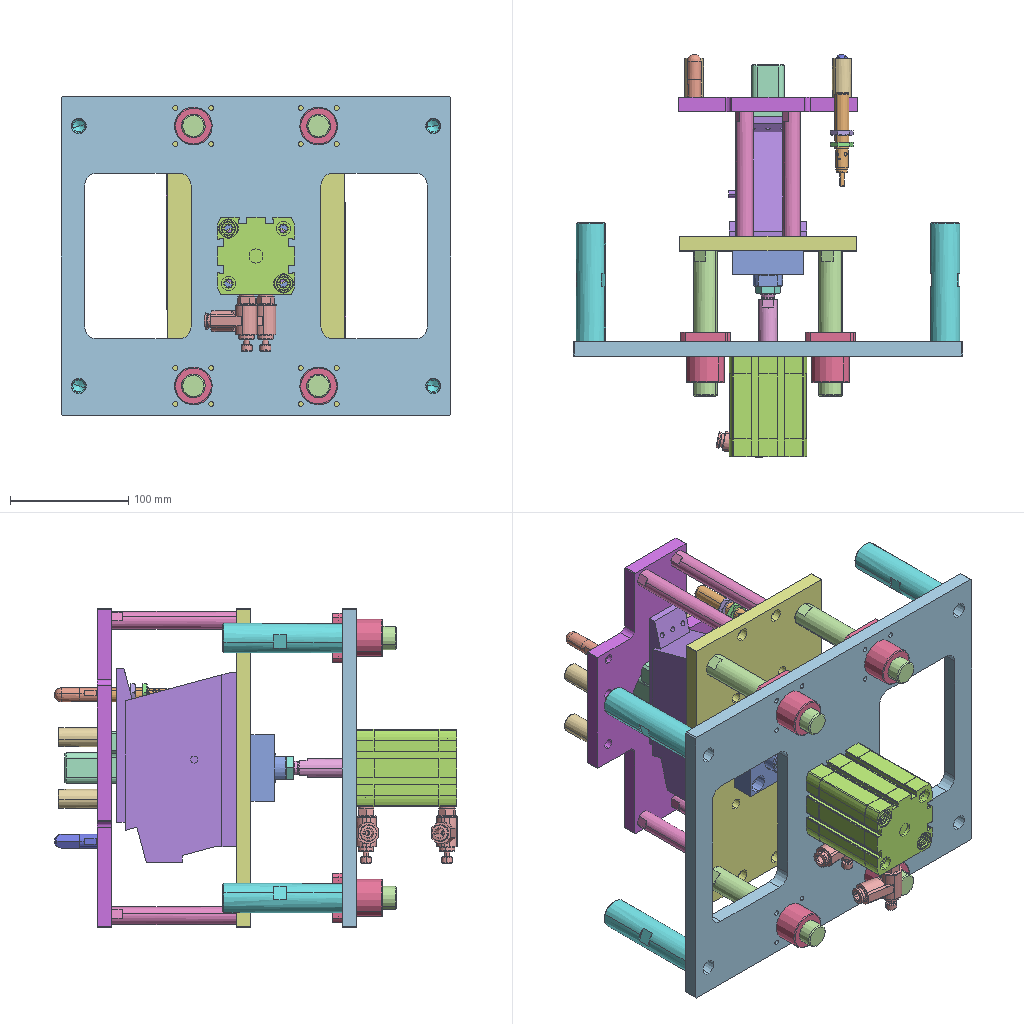Assembly | SolidWorks | 22 different items | 38 placed | box 330 x 341 x 270 mm
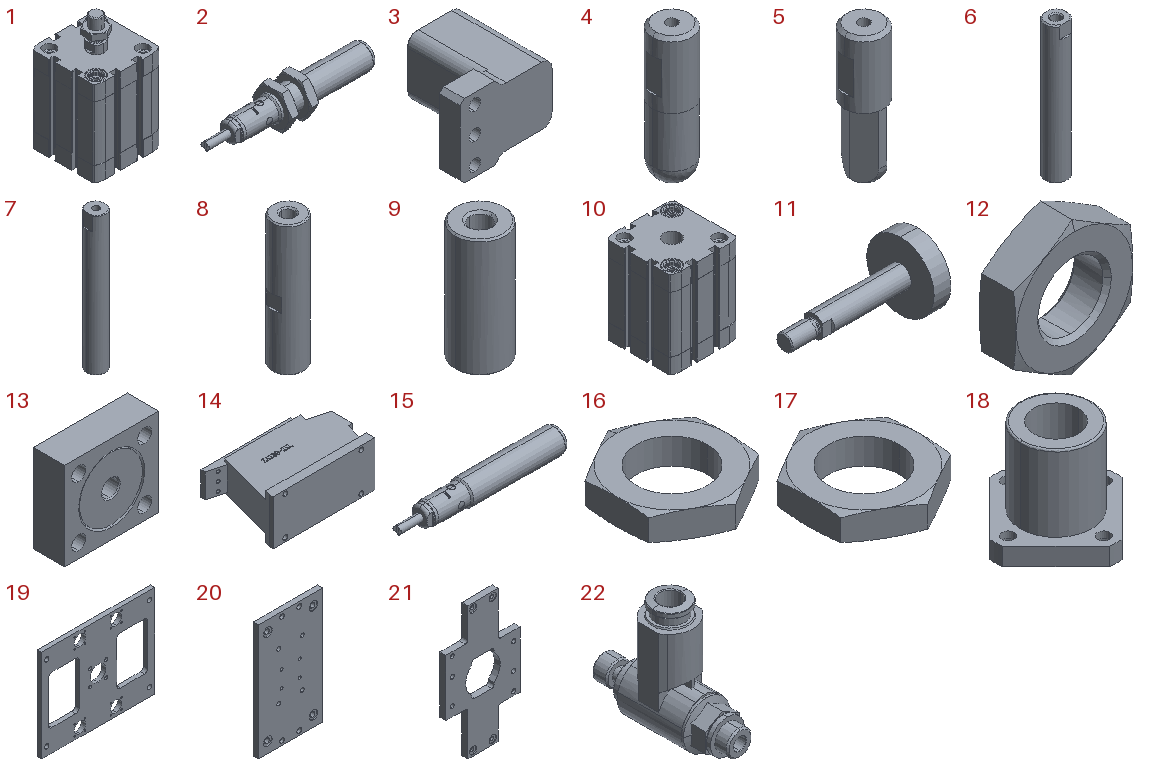Parts list (item | name | quantity | parent item | size | volume | features):
1 | (subassembly) | x1 | - | 65.5 x 65.5 x 115.2 mm | 259589 mm3 | -
2 | (subassembly) | x1 | - | 79.369 x 19.63 x 17 mm | 8383 mm3 | -
3 | - | x1 | - | 44 x 44 x 35 mm | 36722 mm3 | features Chamfer 3, Fillet 2, HoleWzd 2, Extrusion 1, ICE 1
4 | - | x1 | - | 12 x 12 x 41.3 mm | 4237 mm3 | features ICE 2, Chamfer 1, Extrusion 1, HoleWzd 1, Revolution 1
5 | - | x1 | - | 12 x 12 x 41.3 mm | 3482 mm3 | features ICE 3, Chamfer 1, Extrusion 1, HoleWzd 1, Revolution 1
6 | - | x4 | - | 20 x 20 x 125 mm | 37828 mm3 | features BaseBody 1
7 | - | x4 | - | 15 x 15 x 110 mm | 18709 mm3 | features HoleWzd 2, BaseBody 1
8 | - | x4 | - | 25 x 25 x 104 mm | 46673 mm3 | features BaseBody 1, MoveFace 1
9 | - | x4 | - | 16 x 16 x 38 mm | 7208 mm3 | features BaseBody 1
10 | - | x1 | in 1 | 65.5 x 65.5 x 85 mm | 218537 mm3 | features BaseBody 1
11 | - | x1 | in 1 | 98.8 x 50 x 50 mm | 39735 mm3 | features BaseBody 1
12 | - | x1 | in 1 | 19 x 6 x 21.939 mm | 1318 mm3 | features BaseBody 1
13 | - | x1 | - | 60 x 30 x 56 mm | 57044 mm3 | features BaseBody 1
14 | - | x1 | - | 164 x 101.5 x 66 mm | 635286 mm3 | features ICE 6, HoleWzd 2, Extrusion 1
15 | - | x1 | in 2 | 79.369 x 12 x 12 mm | 7140 mm3 | features BaseBody 1
16 | - | x1 | in 2 | 17 x 19.63 x 4 mm | 621.409 mm3 | features BaseBody 1
17 | - | x1 | in 2 | 17 x 19.63 x 4 mm | 621.409 mm3 | features BaseBody 1
18 | - | x4 | - | 54 x 54 x 42 mm | 26435 mm3 | features BaseBody 1
19 | - | x1 | - | 330 x 12 x 270 mm | 691598 mm3 | features ICE 4, HoleWzd 3, Chamfer 1, Extrusion 1
20 | - | x1 | - | 150 x 12 x 270 mm | 470446 mm3 | features HoleWzd 5, ICE 2, Chamfer 1, Extrusion 1
21 | - | x1 | - | 152 x 12 x 270 mm | 265113 mm3 | features ICE 6, HoleWzd 3, Chamfer 1, Extrusion 1, Fillet 1
22 | - | x2 | - | 18 x 52.9 x 44.45 mm | 12907 mm3 | features BaseBody 1
Mates (type | each side: item.copy, entity, surface, feature):
In the top assembly
Width | 20.1 face plane Boss-Extrude1 | 20.1 face plane Boss-Extrude1 | 19.1 face plane Boss-Extrude1 | 19.1 face plane Boss-Extrude1 | 2 times
Width | 21.1 face plane Boss-Extrude1 | 21.1 face plane Boss-Extrude1 | 20.1 face plane Boss-Extrude1 | 20.1 face plane Boss-Extrude1 | 2 times
Concentric | 21.1 face cylinder Cut-Extrude2 | 9.1 face cylinder Input1
Coincident | 21.1 face plane Cut-Extrude2 | 9.1 face plane Input1
Coincident | 21.1 face plane Cut-Extrude2 | 9.2 face plane Input1
Coincident | 21.1 face plane Cut-Extrude2 | 9.3 face plane Input1
Coincident | 21.1 face plane Cut-Extrude2 | 9.4 face plane Input1
Concentric | 21.1 face cylinder Cut-Extrude2 | 9.4 face cylinder Input1
Concentric | 21.1 face cylinder Cut-Extrude2 | 9.3 face cylinder Input1
Concentric | 21.1 face cylinder Cut-Extrude2 | 9.2 face cylinder Input1
Concentric | 21.1 face cylinder Cut-Extrude2 | 4.1 face cylinder Boss-Extrude2
Coincident | 21.1 face plane Cut-Extrude2 | 4.1 face plane Boss-Extrude1
Concentric | 21.1 face cylinder Cut-Extrude5 | 7.1 face cylinder Input1
Coincident | 21.1 face plane Cut-Extrude5 | 7.1 face plane Input1
Coincident | 21.1 face plane Cut-Extrude5 | 7.2 face plane Input1
Coincident | 21.1 face plane Cut-Extrude5 | 7.3 face plane Input1
Coincident | 21.1 face plane Cut-Extrude5 | 7.4 face plane Input1
Concentric | 21.1 face cylinder Cut-Extrude5 | 7.2 face cylinder Input1
Concentric | 21.1 face cylinder Cut-Extrude5 | 7.3 face cylinder Input1
Concentric | 21.1 face cylinder Cut-Extrude5 | 7.4 face cylinder Input1
Coincident | 20.1 face plane Cut-Extrude2 | 7.4 face plane Input1
Coincident | 20.1 face plane Boss-Extrude1 | 13.1 face plane Input1
Concentric | 19.1 face cylinder Cut-Extrude1 | 18.1 face cylinder Input1
Coincident | 19.1 face plane Boss-Extrude1 | 18.1 face plane Input1
Parallel | 19.1 face plane Boss-Extrude1 | 18.1 face plane Input1
Coincident | 19.1 face plane Boss-Extrude1 | 18.2 face plane Input1
Parallel | 19.1 face plane Boss-Extrude1 | 18.2 face plane Input1
Coincident | 19.1 face plane Boss-Extrude1 | 18.3 face plane Input1
Parallel | 19.1 face plane Boss-Extrude1 | 18.3 face plane Input1
Coincident | 19.1 face plane Boss-Extrude1 | 18.4 face plane Input1
Parallel | 19.1 face plane Boss-Extrude1 | 18.4 face plane Input1
Concentric | 19.1 face cylinder Cut-Extrude1 | 18.2 face cylinder Input1
Concentric | 19.1 face cylinder Cut-Extrude1 | 18.3 face cylinder Input1
Concentric | 19.1 face cylinder Cut-Extrude1 | 18.4 face cylinder Input1
Concentric | 18.4 face cylinder Input1 | 6.1 face cylinder Input1
Coincident | 20.1 face plane Cut-Extrude1 | 6.1 face plane Input1
Coincident | 20.1 face plane Cut-Extrude1 | 6.2 face plane Input1
Coincident | 20.1 face plane Cut-Extrude1 | 6.3 face plane Input1
Coincident | 20.1 face plane Cut-Extrude1 | 6.4 face plane Input1
Concentric | 18.1 face cylinder Input1 | 6.2 face cylinder Input1
Concentric | 18.2 face cylinder Input1 | 6.3 face cylinder Input1
Concentric | 18.3 face cylinder Input1 | 6.4 face cylinder Input1
Parallel | 20.1 face plane Boss-Extrude1 | 13.1 face plane Input1
Concentric | 10.1 face cylinder Input1 | 22.1 face cylinder Input1
Coincident | 10.1 face plane Input1 | 22.1 face plane Input1
Coincident | 10.1 face plane Input1 | 22.2 face plane Input1
Concentric | 10.1 face cylinder Input1 | 22.2 face cylinder Input1
Concentric | 13.1 face cylinder Input1 | 11.1 face cylinder Input1
Concentric | 19.1 face cylinder Cut-Extrude2 | 11.1 face cylinder Input1
Coincident | 13.1 face plane Input1 | 12.1 face plane Input1
Parallel | 19.1 face plane Boss-Extrude1 | 10.1 face plane Input1
Coincident | 19.1 face plane Boss-Extrude1 | 10.1 face plane Input1
Concentric | 19.1 face cylinder Cut-Extrude3 | 8.1 face cylinder Input1
Coincident | 19.1 face plane Cut-Extrude3 | 8.1 face plane Input1
Coincident | 19.1 face plane Cut-Extrude3 | 8.2 face plane Input1
Coincident | 19.1 face plane Cut-Extrude3 | 8.3 face plane Input1
Coincident | 19.1 face plane Cut-Extrude3 | 8.4 face plane Input1
Concentric | 19.1 face cylinder Cut-Extrude3 | 8.2 face cylinder Input1
Concentric | 19.1 face cylinder Cut-Extrude3 | 8.3 face cylinder Input1
Concentric | 19.1 face cylinder Cut-Extrude3 | 8.4 face cylinder Input1
Coincident | 20.1 face plane Boss-Extrude1 | 14.1 face plane Boss-Extrude1
Width | 14.1 face plane Boss-Extrude2 | 14.1 face plane Boss-Extrude2 | 20.1 face plane Boss-Extrude1 | 20.1 face plane Boss-Extrude1
Coincident | 3.1 face plane Boss-Extrude1 | 14.1 face plane Boss-Extrude1
Concentric | 3.1 face cylinder M5 Clearance Hole2 | 14.1 face cylinder M5 Tapped Hole1 | 2 times
Concentric | 20.1 face cylinder M8 Clearance Hole1 | 14.1 face cylinder M8 Tapped Hole1
Concentric | 21.1 face cylinder Cut-Extrude2 | 5.1 face cylinder Boss-Extrude2
Coincident | 21.1 face plane Cut-Extrude2 | 5.1 face plane Boss-Extrude1
In subassembly 1
Concentric | 11.2 face cylinder Input1 | 12.2 face cylinder Input1
DistanceDim | 12.2 face plane Input1 | 11.2 face plane Input1
Concentric | 10.2 face cylinder Input1 | 11.2 face cylinder Input1
LimitDistanceDim | 11.2 face plane Input1 | 10.2 face plane Input1